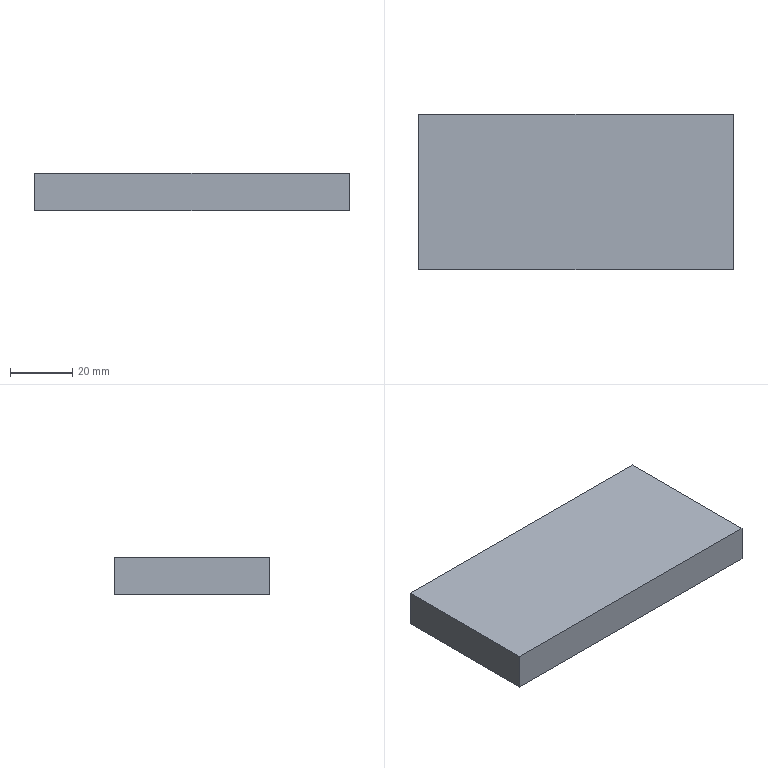Part | SolidWorks | features Extrusion 1 | 1 solid | 6 faces | box 101 x 50 x 12 mm | volume 60600 mm3 | plane 6
STEP:
#1=CARTESIAN_POINT('',(-50.5,25.,-6.));
#2=VERTEX_POINT('',#1);
#3=CARTESIAN_POINT('',(-50.5,-25.,-6.));
#4=VERTEX_POINT('',#3);
#5=CARTESIAN_POINT('',(-50.5,-25.,-6.));
#6=DIRECTION('',(0.,-1.,0.));
#7=VECTOR('',#6,1000.);
#8=LINE('',#5,#7);
#9=EDGE_CURVE('',#2,#4,#8,.T.);
#10=ORIENTED_EDGE('',*,*,#9,.T.);
#11=CARTESIAN_POINT('',(-50.5,-25.,6.));
#12=VERTEX_POINT('',#11);
#13=CARTESIAN_POINT('',(-50.5,-25.,6.));
#14=DIRECTION('',(0.,0.,-1.));
#15=VECTOR('',#14,1000.);
#16=LINE('',#13,#15);
#17=EDGE_CURVE('',#12,#4,#16,.T.);
#18=ORIENTED_EDGE('',*,*,#17,.F.);
#19=CARTESIAN_POINT('',(-50.5,25.,6.));
#20=VERTEX_POINT('',#19);
#21=CARTESIAN_POINT('',(-50.5,-25.,6.));
#22=DIRECTION('',(0.,-1.,0.));
#23=VECTOR('',#22,1000.);
#24=LINE('',#21,#23);
#25=EDGE_CURVE('',#20,#12,#24,.T.);
#26=ORIENTED_EDGE('',*,*,#25,.F.);
#27=CARTESIAN_POINT('',(-50.5,25.,6.));
#28=DIRECTION('',(0.,0.,-1.));
#29=VECTOR('',#28,1000.);
#30=LINE('',#27,#29);
#31=EDGE_CURVE('',#20,#2,#30,.T.);
#32=ORIENTED_EDGE('',*,*,#31,.T.);
#33=EDGE_LOOP('',(#10,#18,#26,#32));
#34=FACE_OUTER_BOUND('',#33,.T.);
#35=CARTESIAN_POINT('',(-50.5,-25.,6.));
#36=DIRECTION('',(1.,0.,0.));
#37=DIRECTION('',(0.,0.,-1.));
#38=AXIS2_PLACEMENT_3D('',#35,#36,#37);
#39=PLANE('',#38);
#40=ADVANCED_FACE('',(#34),#39,.F.);
#41=CARTESIAN_POINT('',(50.5,-25.,-6.));
#42=VERTEX_POINT('',#41);
#43=CARTESIAN_POINT('',(50.5,-25.,-6.));
#44=DIRECTION('',(1.,0.,0.));
#45=VECTOR('',#44,1000.);
#46=LINE('',#43,#45);
#47=EDGE_CURVE('',#4,#42,#46,.T.);
#48=ORIENTED_EDGE('',*,*,#47,.T.);
#49=CARTESIAN_POINT('',(50.5,-25.,6.));
#50=VERTEX_POINT('',#49);
#51=CARTESIAN_POINT('',(50.5,-25.,6.));
#52=DIRECTION('',(0.,0.,-1.));
#53=VECTOR('',#52,1000.);
#54=LINE('',#51,#53);
#55=EDGE_CURVE('',#50,#42,#54,.T.);
#56=ORIENTED_EDGE('',*,*,#55,.F.);
#57=CARTESIAN_POINT('',(50.5,-25.,6.));
#58=DIRECTION('',(1.,0.,0.));
#59=VECTOR('',#58,1000.);
#60=LINE('',#57,#59);
#61=EDGE_CURVE('',#12,#50,#60,.T.);
#62=ORIENTED_EDGE('',*,*,#61,.F.);
#63=ORIENTED_EDGE('',*,*,#17,.T.);
#64=EDGE_LOOP('',(#48,#56,#62,#63));
#65=FACE_OUTER_BOUND('',#64,.T.);
#66=CARTESIAN_POINT('',(50.5,-25.,6.));
#67=DIRECTION('',(0.,1.,0.));
#68=DIRECTION('',(-1.,0.,0.));
#69=AXIS2_PLACEMENT_3D('',#66,#67,#68);
#70=PLANE('',#69);
#71=ADVANCED_FACE('',(#65),#70,.F.);
#72=CARTESIAN_POINT('',(50.5,25.,-6.));
#73=VERTEX_POINT('',#72);
#74=CARTESIAN_POINT('',(50.5,-25.,-6.));
#75=DIRECTION('',(0.,1.,0.));
#76=VECTOR('',#75,1000.);
#77=LINE('',#74,#76);
#78=EDGE_CURVE('',#42,#73,#77,.T.);
#79=ORIENTED_EDGE('',*,*,#78,.T.);
#80=CARTESIAN_POINT('',(50.5,25.,6.));
#81=VERTEX_POINT('',#80);
#82=CARTESIAN_POINT('',(50.5,25.,6.));
#83=DIRECTION('',(0.,0.,-1.));
#84=VECTOR('',#83,1000.);
#85=LINE('',#82,#84);
#86=EDGE_CURVE('',#81,#73,#85,.T.);
#87=ORIENTED_EDGE('',*,*,#86,.F.);
#88=CARTESIAN_POINT('',(50.5,-25.,6.));
#89=DIRECTION('',(0.,1.,0.));
#90=VECTOR('',#89,1000.);
#91=LINE('',#88,#90);
#92=EDGE_CURVE('',#50,#81,#91,.T.);
#93=ORIENTED_EDGE('',*,*,#92,.F.);
#94=ORIENTED_EDGE('',*,*,#55,.T.);
#95=EDGE_LOOP('',(#79,#87,#93,#94));
#96=FACE_OUTER_BOUND('',#95,.T.);
#97=CARTESIAN_POINT('',(50.5,-25.,6.));
#98=DIRECTION('',(-1.,0.,0.));
#99=DIRECTION('',(0.,0.,1.));
#100=AXIS2_PLACEMENT_3D('',#97,#98,#99);
#101=PLANE('',#100);
#102=ADVANCED_FACE('',(#96),#101,.F.);
#103=CARTESIAN_POINT('',(50.5,25.,-6.));
#104=DIRECTION('',(-1.,0.,0.));
#105=VECTOR('',#104,1000.);
#106=LINE('',#103,#105);
#107=EDGE_CURVE('',#73,#2,#106,.T.);
#108=ORIENTED_EDGE('',*,*,#107,.T.);
#109=ORIENTED_EDGE('',*,*,#31,.F.);
#110=CARTESIAN_POINT('',(50.5,25.,6.));
#111=DIRECTION('',(-1.,0.,0.));
#112=VECTOR('',#111,1000.);
#113=LINE('',#110,#112);
#114=EDGE_CURVE('',#81,#20,#113,.T.);
#115=ORIENTED_EDGE('',*,*,#114,.F.);
#116=ORIENTED_EDGE('',*,*,#86,.T.);
#117=EDGE_LOOP('',(#108,#109,#115,#116));
#118=FACE_OUTER_BOUND('',#117,.T.);
#119=CARTESIAN_POINT('',(50.5,25.,6.));
#120=DIRECTION('',(0.,-1.,0.));
#121=DIRECTION('',(1.,0.,0.));
#122=AXIS2_PLACEMENT_3D('',#119,#120,#121);
#123=PLANE('',#122);
#124=ADVANCED_FACE('',(#118),#123,.F.);
#125=ORIENTED_EDGE('',*,*,#25,.T.);
#126=ORIENTED_EDGE('',*,*,#61,.T.);
#127=ORIENTED_EDGE('',*,*,#92,.T.);
#128=ORIENTED_EDGE('',*,*,#114,.T.);
#129=EDGE_LOOP('',(#125,#126,#127,#128));
#130=FACE_OUTER_BOUND('',#129,.T.);
#131=CARTESIAN_POINT('',(0.,0.,6.));
#132=DIRECTION('',(0.,0.,1.));
#133=DIRECTION('',(1.,0.,0.));
#134=AXIS2_PLACEMENT_3D('',#131,#132,#133);
#135=PLANE('',#134);
#136=ADVANCED_FACE('',(#130),#135,.T.);
#137=ORIENTED_EDGE('',*,*,#9,.F.);
#138=ORIENTED_EDGE('',*,*,#107,.F.);
#139=ORIENTED_EDGE('',*,*,#78,.F.);
#140=ORIENTED_EDGE('',*,*,#47,.F.);
#141=EDGE_LOOP('',(#137,#138,#139,#140));
#142=FACE_OUTER_BOUND('',#141,.T.);
#143=CARTESIAN_POINT('',(0.,0.,-6.));
#144=DIRECTION('',(0.,0.,1.));
#145=DIRECTION('',(1.,0.,0.));
#146=AXIS2_PLACEMENT_3D('',#143,#144,#145);
#147=PLANE('',#146);
#148=ADVANCED_FACE('',(#142),#147,.F.);
#149=CLOSED_SHELL('',(#40,#71,#102,#124,#136,#148));
#150=MANIFOLD_SOLID_BREP('',#149);
#151=CARTESIAN_POINT('',(0.,0.,0.));
#152=DIRECTION('',(0.,0.,1.));
#153=DIRECTION('',(1.,0.,0.));
#154=AXIS2_PLACEMENT_3D('',#151,#152,#153);
#155=(LENGTH_UNIT()NAMED_UNIT(*)SI_UNIT(.MILLI.,.METRE.));
#156=UNCERTAINTY_MEASURE_WITH_UNIT(LENGTH_MEASURE(0.00001),#155,'','');
#157=(NAMED_UNIT(*)PLANE_ANGLE_UNIT()SI_UNIT($,.RADIAN.));
#158=(NAMED_UNIT(*)SI_UNIT($,.STERADIAN.)SOLID_ANGLE_UNIT());
#159=(GEOMETRIC_REPRESENTATION_CONTEXT(3)GLOBAL_UNCERTAINTY_ASSIGNED_CONTEXT((#156))GLOBAL_UNIT_ASSIGNED_CONTEXT((#155,#157,#158))REPRESENTATION_CONTEXT('',''));
#160=ADVANCED_BREP_SHAPE_REPRESENTATION('',(#150,#154),#159);